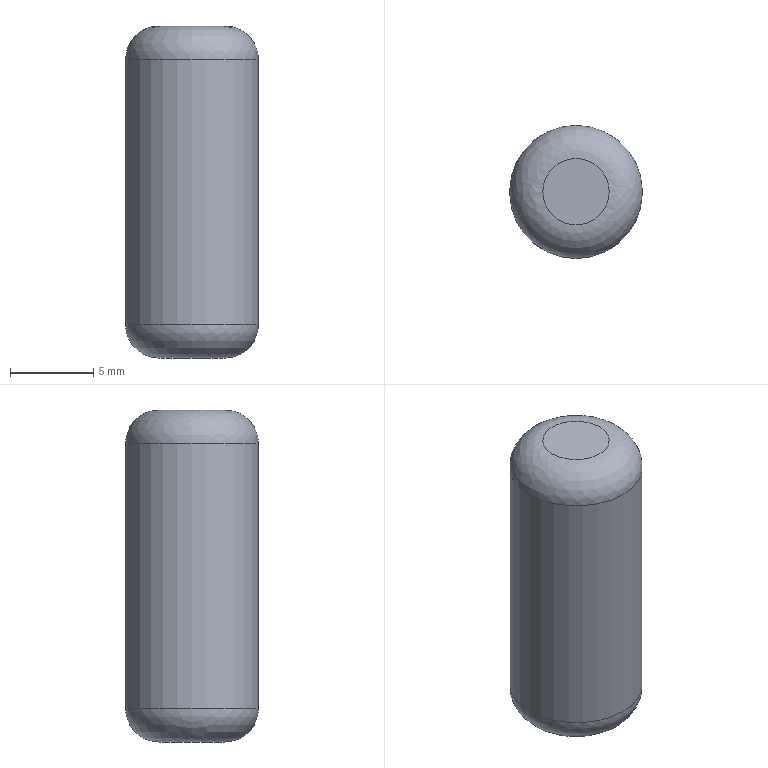Part | STEP file | Tube feed_id1138_x_t | 1 solid | 5 faces | box 8 x 8 x 20 mm | volume 966.7 mm3 | plane 2 | spline 2 | cylinder 1 | commonest cylinder face diameters 8 x1
STEP:
#1=CARTESIAN_POINT('',(0.,0.,0.));
#2=DIRECTION('',(0.,0.,1.));
#3=DIRECTION('',(1.,0.,0.));
#4=AXIS2_PLACEMENT_3D('',#1,#2,#3);
#5=CARTESIAN_POINT('',(-103.,170.056,-122.2));
#6=VERTEX_POINT('',#5);
#7=CARTESIAN_POINT('',(-99.,170.056,-122.2));
#8=DIRECTION('',(0.,0.,1.));
#9=DIRECTION('',(-1.,0.,0.));
#10=AXIS2_PLACEMENT_3D('',#7,#8,#9);
#11=CIRCLE('',#10,4.);
#12=CARTESIAN_POINT('',(-99.,170.056,-124.2));
#13=DIRECTION('',(0.,0.,1.));
#14=DIRECTION('',(1.,0.,0.));
#15=AXIS2_PLACEMENT_3D('',#12,#13,#14);
#16=CYLINDRICAL_SURFACE('',#15,4.);
#17=CARTESIAN_POINT('',(3.142,2.));
#18=DIRECTION('',(1.,0.));
#19=VECTOR('',#18,1.);
#20=LINE('',#17,#19);
#21=(GEOMETRIC_REPRESENTATION_CONTEXT(2)PARAMETRIC_REPRESENTATION_CONTEXT()REPRESENTATION_CONTEXT('',''));
#22=DEFINITIONAL_REPRESENTATION('',(#20),#21);
#23=PCURVE('',#16,#22);
#24=CARTESIAN_POINT('',(-101.,170.056,-124.2));
#25=CARTESIAN_POINT('',(-101.,174.056,-124.2));
#26=CARTESIAN_POINT('',(-97.,174.056,-124.2));
#27=CARTESIAN_POINT('',(-97.,170.056,-124.2));
#28=CARTESIAN_POINT('',(-97.,166.056,-124.2));
#29=CARTESIAN_POINT('',(-101.,166.056,-124.2));
#30=CARTESIAN_POINT('',(-101.,170.056,-124.2));
#31=CARTESIAN_POINT('',(-102.172,170.056,-124.2));
#32=CARTESIAN_POINT('',(-102.172,176.399,-124.2));
#33=CARTESIAN_POINT('',(-95.828,176.399,-124.2));
#34=CARTESIAN_POINT('',(-95.828,170.056,-124.2));
#35=CARTESIAN_POINT('',(-95.828,163.712,-124.2));
#36=CARTESIAN_POINT('',(-102.172,163.712,-124.2));
#37=CARTESIAN_POINT('',(-102.172,170.056,-124.2));
#38=CARTESIAN_POINT('',(-103.,170.056,-123.372));
#39=CARTESIAN_POINT('',(-103.,178.056,-123.372));
#40=CARTESIAN_POINT('',(-95.,178.056,-123.372));
#41=CARTESIAN_POINT('',(-95.,170.056,-123.372));
#42=CARTESIAN_POINT('',(-95.,162.056,-123.372));
#43=CARTESIAN_POINT('',(-103.,162.056,-123.372));
#44=CARTESIAN_POINT('',(-103.,170.056,-123.372));
#45=CARTESIAN_POINT('',(-103.,170.056,-122.2));
#46=CARTESIAN_POINT('',(-103.,178.056,-122.2));
#47=CARTESIAN_POINT('',(-95.,178.056,-122.2));
#48=CARTESIAN_POINT('',(-95.,170.056,-122.2));
#49=CARTESIAN_POINT('',(-95.,162.056,-122.2));
#50=CARTESIAN_POINT('',(-103.,162.056,-122.2));
#51=CARTESIAN_POINT('',(-103.,170.056,-122.2));
#52=(BOUNDED_SURFACE()B_SPLINE_SURFACE(3,3,((#24,#25,#26,#27,#28,#29,#30),(#31,#32,#33,#34,#35,#36,#37),(#38,#39,#40,#41,#42,#43,#44),(#45,#46,#47,#48,#49,#50,#51)),.UNSPECIFIED.,.F.,.T.,.F.)B_SPLINE_SURFACE_WITH_KNOTS((4,4),(1,3,3,3,1),(0.,1.),(-0.5,0.,0.5,1.,1.5),.UNSPECIFIED.)GEOMETRIC_REPRESENTATION_ITEM()RATIONAL_B_SPLINE_SURFACE(((1.,0.3333,0.3333,1.,0.3333,0.3333,1.),(0.8047,0.2682,0.2682,0.8047,0.2682,0.2682,0.8047),(0.8047,0.2682,0.2682,0.8047,0.2682,0.2682,0.8047),(1.,0.3333,0.3333,1.,0.3333,0.3333,1.)))REPRESENTATION_ITEM('')SURFACE());
#53=CARTESIAN_POINT('',(1.,1.));
#54=CARTESIAN_POINT('',(1.,0.9765));
#55=CARTESIAN_POINT('',(1.,0.9351));
#56=CARTESIAN_POINT('',(1.,0.8854));
#57=CARTESIAN_POINT('',(1.,0.8425));
#58=CARTESIAN_POINT('',(1.,0.804));
#59=CARTESIAN_POINT('',(1.,0.7678));
#60=CARTESIAN_POINT('',(1.,0.7322));
#61=CARTESIAN_POINT('',(1.,0.696));
#62=CARTESIAN_POINT('',(1.,0.6575));
#63=CARTESIAN_POINT('',(1.,0.6144));
#64=CARTESIAN_POINT('',(1.,0.5657));
#65=CARTESIAN_POINT('',(1.,0.5));
#66=CARTESIAN_POINT('',(1.,0.4343));
#67=CARTESIAN_POINT('',(1.,0.3856));
#68=CARTESIAN_POINT('',(1.,0.3425));
#69=CARTESIAN_POINT('',(1.,0.304));
#70=CARTESIAN_POINT('',(1.,0.2678));
#71=CARTESIAN_POINT('',(1.,0.2322));
#72=CARTESIAN_POINT('',(1.,0.196));
#73=CARTESIAN_POINT('',(1.,0.1575));
#74=CARTESIAN_POINT('',(1.,0.1146));
#75=CARTESIAN_POINT('',(1.,0.06491));
#76=CARTESIAN_POINT('',(1.,0.02352));
#77=CARTESIAN_POINT('',(1.,0.));
#78=B_SPLINE_CURVE_WITH_KNOTS('',3,(#53,#54,#55,#56,#57,#58,#59,#60,#61,#62,#63,#64,#65,#66,#67,#68,#69,#70,#71,#72,#73,#74,#75,#76,#77),.UNSPECIFIED.,.F.,.F.,(4,1,1,1,1,1,1,1,1,1,1,1,1,1,1,1,1,1,1,1,1,1,4),(0.,0.2856,0.5712,0.8568,1.142,1.428,1.714,1.999,2.285,2.57,2.856,3.142,3.427,3.713,3.998,4.284,4.57,4.855,5.141,5.426,5.712,5.998,6.283),.QUASI_UNIFORM_KNOTS.);
#79=(GEOMETRIC_REPRESENTATION_CONTEXT(2)PARAMETRIC_REPRESENTATION_CONTEXT()REPRESENTATION_CONTEXT('',''));
#80=DEFINITIONAL_REPRESENTATION('',(#78),#79);
#81=PCURVE('',#52,#80);
#82=SURFACE_CURVE('',#11,(#23,#81),.PCURVE_S1.);
#83=EDGE_CURVE('',#6,#6,#82,.T.);
#84=ORIENTED_EDGE('',*,*,#83,.T.);
#85=CARTESIAN_POINT('',(-103.,170.056,-106.2));
#86=VERTEX_POINT('',#85);
#87=CARTESIAN_POINT('',(-103.,170.056,-122.2));
#88=CARTESIAN_POINT('',(-103.,170.056,-106.2));
#89=B_SPLINE_CURVE_WITH_KNOTS('',1,(#87,#88),.UNSPECIFIED.,.F.,.F.,(2,2),(2.,18.),.PIECEWISE_BEZIER_KNOTS.);
#90=CARTESIAN_POINT('',(9.425,0.));
#91=DIRECTION('',(0.,1.));
#92=VECTOR('',#91,1.);
#93=LINE('',#90,#92);
#94=(GEOMETRIC_REPRESENTATION_CONTEXT(2)PARAMETRIC_REPRESENTATION_CONTEXT()REPRESENTATION_CONTEXT('',''));
#95=DEFINITIONAL_REPRESENTATION('',(#93),#94);
#96=PCURVE('',#16,#95);
#97=CARTESIAN_POINT('',(3.142,0.));
#98=DIRECTION('',(0.,1.));
#99=VECTOR('',#98,1.);
#100=LINE('',#97,#99);
#101=(GEOMETRIC_REPRESENTATION_CONTEXT(2)PARAMETRIC_REPRESENTATION_CONTEXT()REPRESENTATION_CONTEXT('',''));
#102=DEFINITIONAL_REPRESENTATION('',(#100),#101);
#103=PCURVE('',#16,#102);
#104=SEAM_CURVE('',#89,(#96,#103),.PCURVE_S1.);
#105=EDGE_CURVE('',#6,#86,#104,.T.);
#106=ORIENTED_EDGE('',*,*,#105,.T.);
#107=CARTESIAN_POINT('',(-99.,170.056,-106.2));
#108=DIRECTION('',(0.,0.,-1.));
#109=DIRECTION('',(-1.,0.,0.));
#110=AXIS2_PLACEMENT_3D('',#107,#108,#109);
#111=CIRCLE('',#110,4.);
#112=CARTESIAN_POINT('',(9.425,18.));
#113=DIRECTION('',(-1.,0.));
#114=VECTOR('',#113,1.);
#115=LINE('',#112,#114);
#116=(GEOMETRIC_REPRESENTATION_CONTEXT(2)PARAMETRIC_REPRESENTATION_CONTEXT()REPRESENTATION_CONTEXT('',''));
#117=DEFINITIONAL_REPRESENTATION('',(#115),#116);
#118=PCURVE('',#16,#117);
#119=CARTESIAN_POINT('',(-103.,170.056,-106.2));
#120=CARTESIAN_POINT('',(-103.,178.056,-106.2));
#121=CARTESIAN_POINT('',(-95.,178.056,-106.2));
#122=CARTESIAN_POINT('',(-95.,170.056,-106.2));
#123=CARTESIAN_POINT('',(-95.,162.056,-106.2));
#124=CARTESIAN_POINT('',(-103.,162.056,-106.2));
#125=CARTESIAN_POINT('',(-103.,170.056,-106.2));
#126=CARTESIAN_POINT('',(-103.,170.056,-105.028));
#127=CARTESIAN_POINT('',(-103.,178.056,-105.028));
#128=CARTESIAN_POINT('',(-95.,178.056,-105.028));
#129=CARTESIAN_POINT('',(-95.,170.056,-105.028));
#130=CARTESIAN_POINT('',(-95.,162.056,-105.028));
#131=CARTESIAN_POINT('',(-103.,162.056,-105.028));
#132=CARTESIAN_POINT('',(-103.,170.056,-105.028));
#133=CARTESIAN_POINT('',(-102.172,170.056,-104.2));
#134=CARTESIAN_POINT('',(-102.172,176.399,-104.2));
#135=CARTESIAN_POINT('',(-95.828,176.399,-104.2));
#136=CARTESIAN_POINT('',(-95.828,170.056,-104.2));
#137=CARTESIAN_POINT('',(-95.828,163.712,-104.2));
#138=CARTESIAN_POINT('',(-102.172,163.712,-104.2));
#139=CARTESIAN_POINT('',(-102.172,170.056,-104.2));
#140=CARTESIAN_POINT('',(-101.,170.056,-104.2));
#141=CARTESIAN_POINT('',(-101.,174.056,-104.2));
#142=CARTESIAN_POINT('',(-97.,174.056,-104.2));
#143=CARTESIAN_POINT('',(-97.,170.056,-104.2));
#144=CARTESIAN_POINT('',(-97.,166.056,-104.2));
#145=CARTESIAN_POINT('',(-101.,166.056,-104.2));
#146=CARTESIAN_POINT('',(-101.,170.056,-104.2));
#147=(BOUNDED_SURFACE()B_SPLINE_SURFACE(3,3,((#119,#120,#121,#122,#123,#124,#125),(#126,#127,#128,#129,#130,#131,#132),(#133,#134,#135,#136,#137,#138,#139),(#140,#141,#142,#143,#144,#145,#146)),.UNSPECIFIED.,.F.,.T.,.F.)B_SPLINE_SURFACE_WITH_KNOTS((4,4),(1,3,3,3,1),(0.,1.),(-0.5,0.,0.5,1.,1.5),.UNSPECIFIED.)GEOMETRIC_REPRESENTATION_ITEM()RATIONAL_B_SPLINE_SURFACE(((1.,0.3333,0.3333,1.,0.3333,0.3333,1.),(0.8047,0.2682,0.2682,0.8047,0.2682,0.2682,0.8047),(0.8047,0.2682,0.2682,0.8047,0.2682,0.2682,0.8047),(1.,0.3333,0.3333,1.,0.3333,0.3333,1.)))REPRESENTATION_ITEM('')SURFACE());
#148=CARTESIAN_POINT('',(0.,0.));
#149=CARTESIAN_POINT('',(0.,0.02352));
#150=CARTESIAN_POINT('',(0.,0.06491));
#151=CARTESIAN_POINT('',(0.,0.1146));
#152=CARTESIAN_POINT('',(0.,0.1575));
#153=CARTESIAN_POINT('',(0.,0.196));
#154=CARTESIAN_POINT('',(0.,0.2322));
#155=CARTESIAN_POINT('',(0.,0.2678));
#156=CARTESIAN_POINT('',(0.,0.304));
#157=CARTESIAN_POINT('',(0.,0.3425));
#158=CARTESIAN_POINT('',(0.,0.3856));
#159=CARTESIAN_POINT('',(0.,0.4343));
#160=CARTESIAN_POINT('',(0.,0.5));
#161=CARTESIAN_POINT('',(0.,0.5657));
#162=CARTESIAN_POINT('',(0.,0.6144));
#163=CARTESIAN_POINT('',(0.,0.6575));
#164=CARTESIAN_POINT('',(0.,0.696));
#165=CARTESIAN_POINT('',(0.,0.7322));
#166=CARTESIAN_POINT('',(0.,0.7678));
#167=CARTESIAN_POINT('',(0.,0.804));
#168=CARTESIAN_POINT('',(0.,0.8425));
#169=CARTESIAN_POINT('',(0.,0.8854));
#170=CARTESIAN_POINT('',(0.,0.9351));
#171=CARTESIAN_POINT('',(0.,0.9765));
#172=CARTESIAN_POINT('',(0.,1.));
#173=B_SPLINE_CURVE_WITH_KNOTS('',3,(#148,#149,#150,#151,#152,#153,#154,#155,#156,#157,#158,#159,#160,#161,#162,#163,#164,#165,#166,#167,#168,#169,#170,#171,#172),.UNSPECIFIED.,.F.,.F.,(4,1,1,1,1,1,1,1,1,1,1,1,1,1,1,1,1,1,1,1,1,1,4),(0.,0.2856,0.5712,0.8568,1.142,1.428,1.714,1.999,2.285,2.57,2.856,3.142,3.427,3.713,3.998,4.284,4.57,4.855,5.141,5.426,5.712,5.998,6.283),.QUASI_UNIFORM_KNOTS.);
#174=(GEOMETRIC_REPRESENTATION_CONTEXT(2)PARAMETRIC_REPRESENTATION_CONTEXT()REPRESENTATION_CONTEXT('',''));
#175=DEFINITIONAL_REPRESENTATION('',(#173),#174);
#176=PCURVE('',#147,#175);
#177=SURFACE_CURVE('',#111,(#118,#176),.PCURVE_S1.);
#178=EDGE_CURVE('',#86,#86,#177,.T.);
#179=ORIENTED_EDGE('',*,*,#178,.T.);
#180=ORIENTED_EDGE('',*,*,#105,.F.);
#181=EDGE_LOOP('',(#84,#106,#179,#180));
#182=FACE_BOUND('',#181,.T.);
#183=ADVANCED_FACE('',(#182),#16,.T.);
#184=CARTESIAN_POINT('',(-101.,170.056,-124.2));
#185=VERTEX_POINT('',#184);
#186=CARTESIAN_POINT('',(-99.,170.056,-124.2));
#187=DIRECTION('',(0.,0.,-1.));
#188=DIRECTION('',(-1.,0.,0.));
#189=AXIS2_PLACEMENT_3D('',#186,#187,#188);
#190=CIRCLE('',#189,2.);
#191=CARTESIAN_POINT('',(-99.,170.056,-124.2));
#192=DIRECTION('',(0.,0.,-1.));
#193=DIRECTION('',(-1.,0.,0.));
#194=AXIS2_PLACEMENT_3D('',#191,#192,#193);
#195=PLANE('',#194);
#196=CARTESIAN_POINT('',(0.,0.));
#197=DIRECTION('',(1.,0.));
#198=AXIS2_PLACEMENT_2D('',#196,#197);
#199=CIRCLE('',#198,2.);
#200=(GEOMETRIC_REPRESENTATION_CONTEXT(2)PARAMETRIC_REPRESENTATION_CONTEXT()REPRESENTATION_CONTEXT('',''));
#201=DEFINITIONAL_REPRESENTATION('',(#199),#200);
#202=PCURVE('',#195,#201);
#203=CARTESIAN_POINT('',(0.,0.));
#204=CARTESIAN_POINT('',(0.,0.02352));
#205=CARTESIAN_POINT('',(0.,0.06491));
#206=CARTESIAN_POINT('',(0.,0.1146));
#207=CARTESIAN_POINT('',(0.,0.1575));
#208=CARTESIAN_POINT('',(0.,0.196));
#209=CARTESIAN_POINT('',(0.,0.2322));
#210=CARTESIAN_POINT('',(0.,0.2678));
#211=CARTESIAN_POINT('',(0.,0.304));
#212=CARTESIAN_POINT('',(0.,0.3425));
#213=CARTESIAN_POINT('',(0.,0.3856));
#214=CARTESIAN_POINT('',(0.,0.4343));
#215=CARTESIAN_POINT('',(0.,0.5));
#216=CARTESIAN_POINT('',(0.,0.5657));
#217=CARTESIAN_POINT('',(0.,0.6144));
#218=CARTESIAN_POINT('',(0.,0.6575));
#219=CARTESIAN_POINT('',(0.,0.696));
#220=CARTESIAN_POINT('',(0.,0.7322));
#221=CARTESIAN_POINT('',(0.,0.7678));
#222=CARTESIAN_POINT('',(0.,0.804));
#223=CARTESIAN_POINT('',(0.,0.8425));
#224=CARTESIAN_POINT('',(0.,0.8854));
#225=CARTESIAN_POINT('',(0.,0.9351));
#226=CARTESIAN_POINT('',(0.,0.9765));
#227=CARTESIAN_POINT('',(0.,1.));
#228=B_SPLINE_CURVE_WITH_KNOTS('',3,(#203,#204,#205,#206,#207,#208,#209,#210,#211,#212,#213,#214,#215,#216,#217,#218,#219,#220,#221,#222,#223,#224,#225,#226,#227),.UNSPECIFIED.,.F.,.F.,(4,1,1,1,1,1,1,1,1,1,1,1,1,1,1,1,1,1,1,1,1,1,4),(0.,0.2856,0.5712,0.8568,1.142,1.428,1.714,1.999,2.285,2.57,2.856,3.142,3.427,3.713,3.998,4.284,4.57,4.855,5.141,5.426,5.712,5.998,6.283),.QUASI_UNIFORM_KNOTS.);
#229=(GEOMETRIC_REPRESENTATION_CONTEXT(2)PARAMETRIC_REPRESENTATION_CONTEXT()REPRESENTATION_CONTEXT('',''));
#230=DEFINITIONAL_REPRESENTATION('',(#228),#229);
#231=PCURVE('',#52,#230);
#232=SURFACE_CURVE('',#190,(#202,#231),.PCURVE_S1.);
#233=EDGE_CURVE('',#185,#185,#232,.T.);
#234=ORIENTED_EDGE('',*,*,#233,.T.);
#235=EDGE_LOOP('',(#234));
#236=FACE_BOUND('',#235,.T.);
#237=ADVANCED_FACE('',(#236),#195,.T.);
#238=CARTESIAN_POINT('',(-101.,170.056,-104.2));
#239=VERTEX_POINT('',#238);
#240=CARTESIAN_POINT('',(-99.,170.056,-104.2));
#241=DIRECTION('',(0.,0.,1.));
#242=DIRECTION('',(-1.,0.,0.));
#243=AXIS2_PLACEMENT_3D('',#240,#241,#242);
#244=CIRCLE('',#243,2.);
#245=CARTESIAN_POINT('',(-99.,170.056,-104.2));
#246=DIRECTION('',(0.,0.,-1.));
#247=DIRECTION('',(-1.,0.,0.));
#248=AXIS2_PLACEMENT_3D('',#245,#246,#247);
#249=PLANE('',#248);
#250=CARTESIAN_POINT('',(2.,0.));
#251=CARTESIAN_POINT('',(2.,-3.464));
#252=CARTESIAN_POINT('',(-1.,-1.732));
#253=CARTESIAN_POINT('',(-4.,0.));
#254=CARTESIAN_POINT('',(-1.,1.732));
#255=CARTESIAN_POINT('',(2.,3.464));
#256=CARTESIAN_POINT('',(2.,0.));
#257=(BOUNDED_CURVE()B_SPLINE_CURVE(2,(#250,#251,#252,#253,#254,#255,#256),.UNSPECIFIED.,.T.,.F.)B_SPLINE_CURVE_WITH_KNOTS((1,2,2,2,2,1),(-2.094,0.,2.094,4.189,6.283,8.378),.UNSPECIFIED.)CURVE()GEOMETRIC_REPRESENTATION_ITEM()RATIONAL_B_SPLINE_CURVE((1.,0.5,1.,0.5,1.,0.5,1.))REPRESENTATION_ITEM(''));
#258=(GEOMETRIC_REPRESENTATION_CONTEXT(2)PARAMETRIC_REPRESENTATION_CONTEXT()REPRESENTATION_CONTEXT('',''));
#259=DEFINITIONAL_REPRESENTATION('',(#257),#258);
#260=PCURVE('',#249,#259);
#261=CARTESIAN_POINT('',(1.,1.));
#262=CARTESIAN_POINT('',(1.,0.9765));
#263=CARTESIAN_POINT('',(1.,0.9351));
#264=CARTESIAN_POINT('',(1.,0.8854));
#265=CARTESIAN_POINT('',(1.,0.8425));
#266=CARTESIAN_POINT('',(1.,0.804));
#267=CARTESIAN_POINT('',(1.,0.7678));
#268=CARTESIAN_POINT('',(1.,0.7322));
#269=CARTESIAN_POINT('',(1.,0.696));
#270=CARTESIAN_POINT('',(1.,0.6575));
#271=CARTESIAN_POINT('',(1.,0.6144));
#272=CARTESIAN_POINT('',(1.,0.5657));
#273=CARTESIAN_POINT('',(1.,0.5));
#274=CARTESIAN_POINT('',(1.,0.4343));
#275=CARTESIAN_POINT('',(1.,0.3856));
#276=CARTESIAN_POINT('',(1.,0.3425));
#277=CARTESIAN_POINT('',(1.,0.304));
#278=CARTESIAN_POINT('',(1.,0.2678));
#279=CARTESIAN_POINT('',(1.,0.2322));
#280=CARTESIAN_POINT('',(1.,0.196));
#281=CARTESIAN_POINT('',(1.,0.1575));
#282=CARTESIAN_POINT('',(1.,0.1146));
#283=CARTESIAN_POINT('',(1.,0.06491));
#284=CARTESIAN_POINT('',(1.,0.02352));
#285=CARTESIAN_POINT('',(1.,0.));
#286=B_SPLINE_CURVE_WITH_KNOTS('',3,(#261,#262,#263,#264,#265,#266,#267,#268,#269,#270,#271,#272,#273,#274,#275,#276,#277,#278,#279,#280,#281,#282,#283,#284,#285),.UNSPECIFIED.,.F.,.F.,(4,1,1,1,1,1,1,1,1,1,1,1,1,1,1,1,1,1,1,1,1,1,4),(0.,0.2856,0.5712,0.8568,1.142,1.428,1.714,1.999,2.285,2.57,2.856,3.142,3.427,3.713,3.998,4.284,4.57,4.855,5.141,5.426,5.712,5.998,6.283),.QUASI_UNIFORM_KNOTS.);
#287=(GEOMETRIC_REPRESENTATION_CONTEXT(2)PARAMETRIC_REPRESENTATION_CONTEXT()REPRESENTATION_CONTEXT('',''));
#288=DEFINITIONAL_REPRESENTATION('',(#286),#287);
#289=PCURVE('',#147,#288);
#290=SURFACE_CURVE('',#244,(#260,#289),.PCURVE_S1.);
#291=EDGE_CURVE('',#239,#239,#290,.T.);
#292=ORIENTED_EDGE('',*,*,#291,.T.);
#293=EDGE_LOOP('',(#292));
#294=FACE_BOUND('',#293,.T.);
#295=ADVANCED_FACE('',(#294),#249,.F.);
#296=ORIENTED_EDGE('',*,*,#83,.F.);
#297=CARTESIAN_POINT('',(-101.,170.056,-124.2));
#298=CARTESIAN_POINT('',(-102.172,170.056,-124.2));
#299=CARTESIAN_POINT('',(-103.,170.056,-123.372));
#300=CARTESIAN_POINT('',(-103.,170.056,-122.2));
#301=(BOUNDED_CURVE()B_SPLINE_CURVE(3,(#297,#298,#299,#300),.UNSPECIFIED.,.F.,.F.)B_SPLINE_CURVE_WITH_KNOTS((4,4),(0.,1.),.PIECEWISE_BEZIER_KNOTS.)CURVE()GEOMETRIC_REPRESENTATION_ITEM()RATIONAL_B_SPLINE_CURVE((1.,0.8047,0.8047,1.))REPRESENTATION_ITEM(''));
#302=CARTESIAN_POINT('',(0.,1.));
#303=DIRECTION('',(1.,0.));
#304=VECTOR('',#303,1.);
#305=LINE('',#302,#304);
#306=(GEOMETRIC_REPRESENTATION_CONTEXT(2)PARAMETRIC_REPRESENTATION_CONTEXT()REPRESENTATION_CONTEXT('',''));
#307=DEFINITIONAL_REPRESENTATION('',(#305),#306);
#308=PCURVE('',#52,#307);
#309=CARTESIAN_POINT('',(0.,0.));
#310=DIRECTION('',(1.,0.));
#311=VECTOR('',#310,1.);
#312=LINE('',#309,#311);
#313=(GEOMETRIC_REPRESENTATION_CONTEXT(2)PARAMETRIC_REPRESENTATION_CONTEXT()REPRESENTATION_CONTEXT('',''));
#314=DEFINITIONAL_REPRESENTATION('',(#312),#313);
#315=PCURVE('',#52,#314);
#316=SEAM_CURVE('',#301,(#308,#315),.PCURVE_S1.);
#317=EDGE_CURVE('',#185,#6,#316,.T.);
#318=ORIENTED_EDGE('',*,*,#317,.F.);
#319=ORIENTED_EDGE('',*,*,#233,.F.);
#320=ORIENTED_EDGE('',*,*,#317,.T.);
#321=EDGE_LOOP('',(#296,#318,#319,#320));
#322=FACE_BOUND('',#321,.T.);
#323=ADVANCED_FACE('',(#322),#52,.T.);
#324=ORIENTED_EDGE('',*,*,#291,.F.);
#325=CARTESIAN_POINT('',(-103.,170.056,-106.2));
#326=CARTESIAN_POINT('',(-103.,170.056,-105.028));
#327=CARTESIAN_POINT('',(-102.172,170.056,-104.2));
#328=CARTESIAN_POINT('',(-101.,170.056,-104.2));
#329=(BOUNDED_CURVE()B_SPLINE_CURVE(3,(#325,#326,#327,#328),.UNSPECIFIED.,.F.,.F.)B_SPLINE_CURVE_WITH_KNOTS((4,4),(0.,1.),.PIECEWISE_BEZIER_KNOTS.)CURVE()GEOMETRIC_REPRESENTATION_ITEM()RATIONAL_B_SPLINE_CURVE((1.,0.8047,0.8047,1.))REPRESENTATION_ITEM(''));
#330=CARTESIAN_POINT('',(0.,1.));
#331=DIRECTION('',(1.,0.));
#332=VECTOR('',#331,1.);
#333=LINE('',#330,#332);
#334=(GEOMETRIC_REPRESENTATION_CONTEXT(2)PARAMETRIC_REPRESENTATION_CONTEXT()REPRESENTATION_CONTEXT('',''));
#335=DEFINITIONAL_REPRESENTATION('',(#333),#334);
#336=PCURVE('',#147,#335);
#337=CARTESIAN_POINT('',(0.,0.));
#338=DIRECTION('',(1.,0.));
#339=VECTOR('',#338,1.);
#340=LINE('',#337,#339);
#341=(GEOMETRIC_REPRESENTATION_CONTEXT(2)PARAMETRIC_REPRESENTATION_CONTEXT()REPRESENTATION_CONTEXT('',''));
#342=DEFINITIONAL_REPRESENTATION('',(#340),#341);
#343=PCURVE('',#147,#342);
#344=SEAM_CURVE('',#329,(#336,#343),.PCURVE_S1.);
#345=EDGE_CURVE('',#86,#239,#344,.T.);
#346=ORIENTED_EDGE('',*,*,#345,.F.);
#347=ORIENTED_EDGE('',*,*,#178,.F.);
#348=ORIENTED_EDGE('',*,*,#345,.T.);
#349=EDGE_LOOP('',(#324,#346,#347,#348));
#350=FACE_BOUND('',#349,.T.);
#351=ADVANCED_FACE('',(#350),#147,.T.);
#352=CLOSED_SHELL('',(#183,#237,#295,#323,#351));
#353=MANIFOLD_SOLID_BREP('',#352);
#354=(LENGTH_UNIT()NAMED_UNIT(*)SI_UNIT(.MILLI.,.METRE.));
#355=UNCERTAINTY_MEASURE_WITH_UNIT(LENGTH_MEASURE(0.00001),#354,'','');
#356=(NAMED_UNIT(*)PLANE_ANGLE_UNIT()SI_UNIT($,.RADIAN.));
#357=(NAMED_UNIT(*)SI_UNIT($,.STERADIAN.)SOLID_ANGLE_UNIT());
#358=(GEOMETRIC_REPRESENTATION_CONTEXT(3)GLOBAL_UNCERTAINTY_ASSIGNED_CONTEXT((#355))GLOBAL_UNIT_ASSIGNED_CONTEXT((#354,#356,#357))REPRESENTATION_CONTEXT('',''));
#359=ADVANCED_BREP_SHAPE_REPRESENTATION('',(#4,#353),#358);